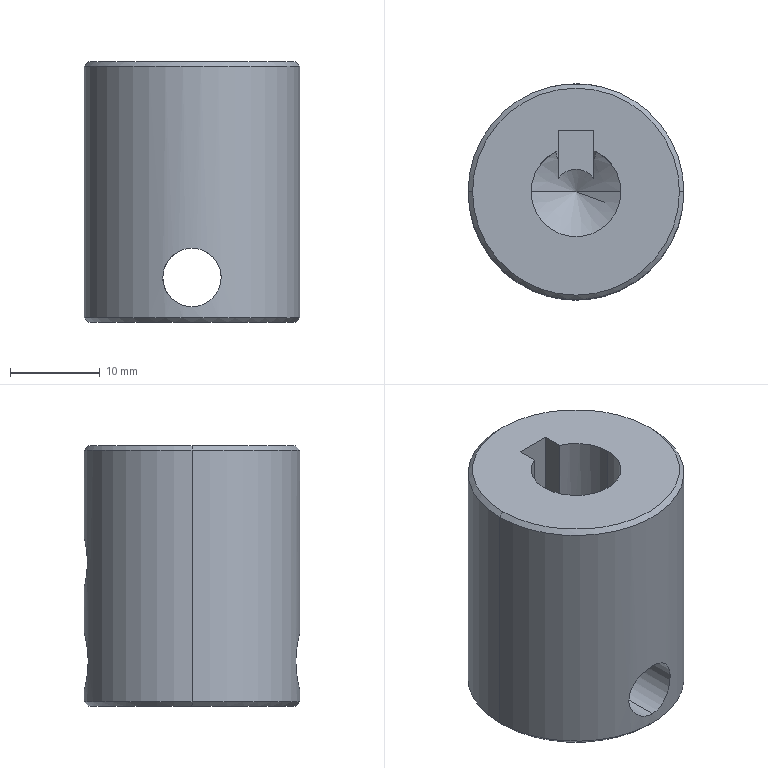Part | SolidWorks | features ICE 3, Chamfer 2, Extrusion 1, HoleWzd 1 | 1 solid | 27 faces | box 24 x 24 x 29 mm | volume 10899 mm3 | plane 10 | cylinder 9 | cone 6 | spline 2 | commonest cylinder face diameters 10 x3 5 x2 6.5 x2 24 x2